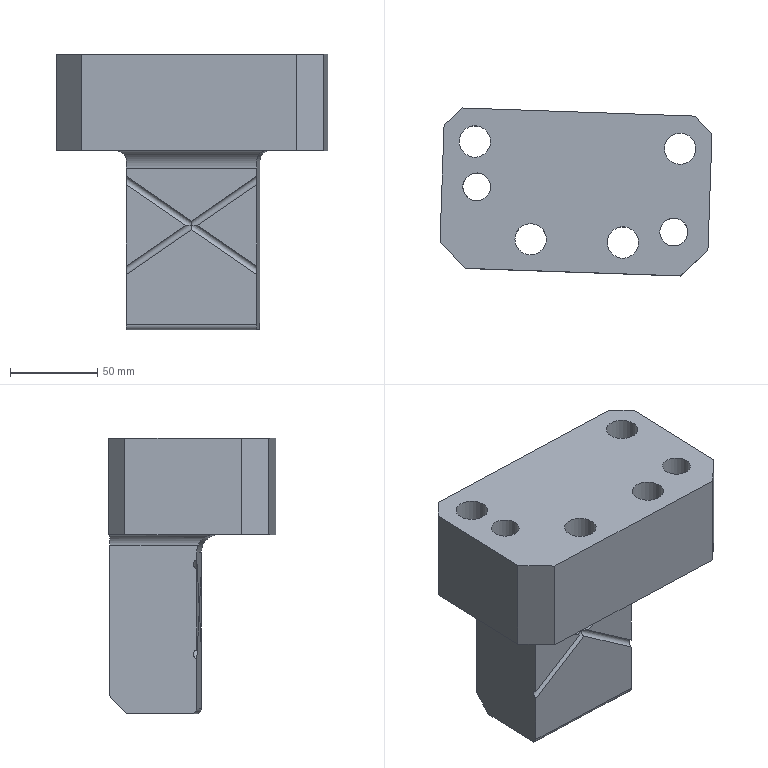Part | NX | features UB-11 2 | 1 solid | 54 faces | box 156.244 x 96.445 x 158.5 mm | volume 1045715 mm3 | plane 26 | cylinder 26 | cone 2 | commonest cylinder face diameters 18 x6 4 x4 26 x4 6 x3 10.3 x2 12 x2